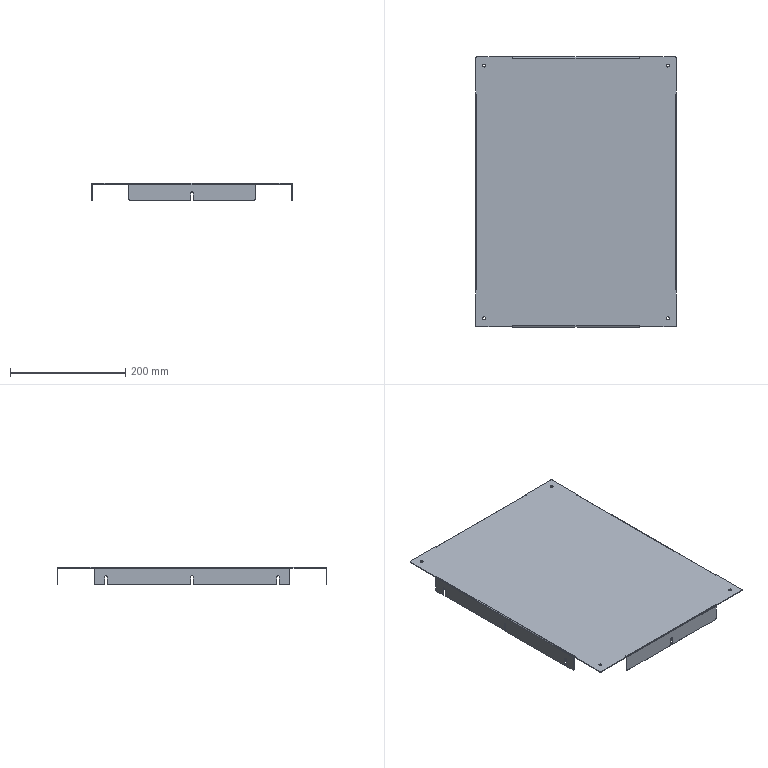Part | STEP file | 1 solid | 128 faces | box 349 x 469 x 30 mm | volume 233516 mm3 | plane 86 | cylinder 42 | commonest cylinder face diameters 4.5 x14 4 x12 5 x8 1.2 x4 3.6 x4